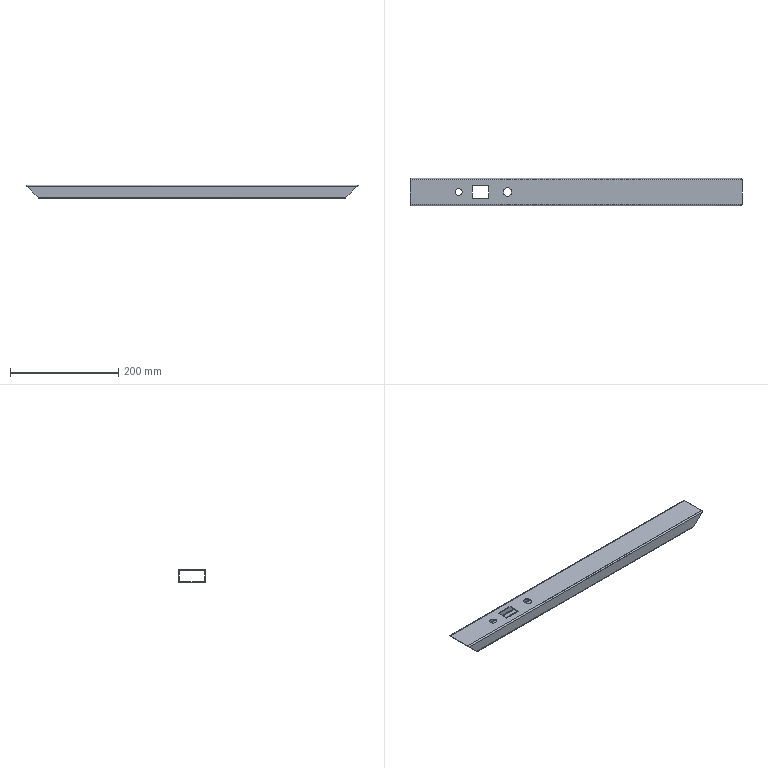Part | STEP file | 7100502 | 1 solid | 31 faces | box 613 x 50 x 25 mm | volume 116984 mm3 | plane 20 | cylinder 11 | commonest cylinder face diameters 2 x4 5 x4 15.8 x2 13 x1